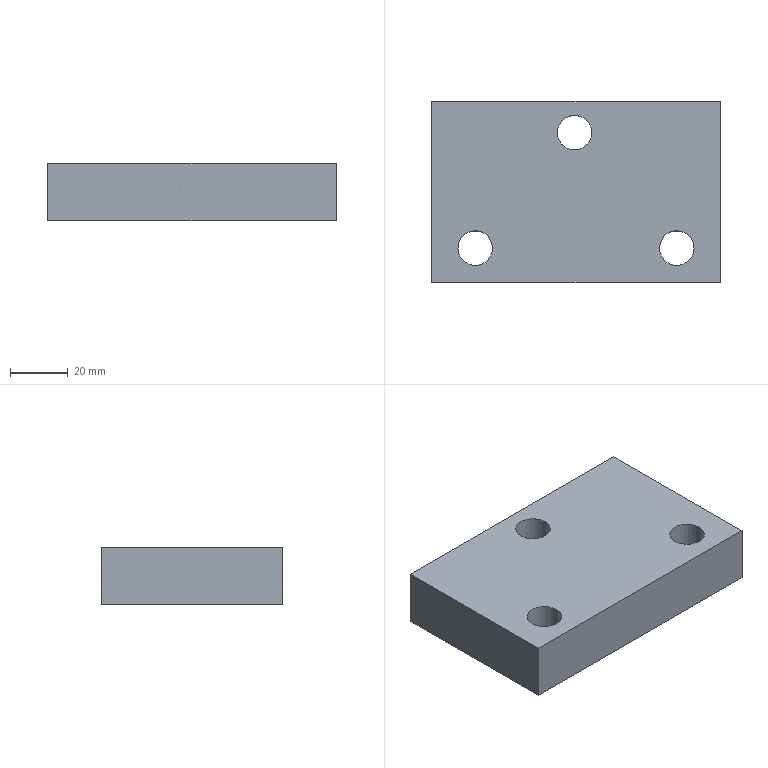Part | STEP file | cu dao nhan | 1 solid | 18 faces | box 100 x 63 x 20 mm | volume 110399 mm3 | plane 10 | cylinder 8 | commonest cylinder face diameters 12 x6 6 x2
STEP:
#1=CARTESIAN_POINT('',(0.,0.,0.));
#2=DIRECTION('',(0.,0.,1.));
#3=DIRECTION('',(1.,0.,0.));
#4=AXIS2_PLACEMENT_3D('',#1,#2,#3);
#5=CARTESIAN_POINT('',(55.5,52.1,5.));
#6=VERTEX_POINT('',#5);
#7=CARTESIAN_POINT('',(55.5,52.1,20.));
#8=VERTEX_POINT('',#7);
#9=CARTESIAN_POINT('',(55.5,52.1,-99.871));
#10=DIRECTION('',(0.,0.,1.));
#11=VECTOR('',#10,1.);
#12=LINE('',#9,#11);
#13=CARTESIAN_POINT('',(49.5,52.1,-99.871));
#14=DIRECTION('',(0.,0.,1.));
#15=DIRECTION('',(1.,0.,0.));
#16=AXIS2_PLACEMENT_3D('',#13,#14,#15);
#17=CYLINDRICAL_SURFACE('',#16,6.);
#18=CARTESIAN_POINT('',(6.283,0.));
#19=DIRECTION('',(0.,1.));
#20=VECTOR('',#19,1.);
#21=LINE('',#18,#20);
#22=(GEOMETRIC_REPRESENTATION_CONTEXT(2)PARAMETRIC_REPRESENTATION_CONTEXT()REPRESENTATION_CONTEXT('',''));
#23=DEFINITIONAL_REPRESENTATION('',(#21),#22);
#24=PCURVE('',#17,#23);
#25=CARTESIAN_POINT('',(49.5,52.1,-99.871));
#26=DIRECTION('',(0.,0.,1.));
#27=DIRECTION('',(1.,0.,0.));
#28=AXIS2_PLACEMENT_3D('',#25,#26,#27);
#29=CYLINDRICAL_SURFACE('',#28,6.);
#30=CARTESIAN_POINT('',(0.,0.));
#31=DIRECTION('',(0.,1.));
#32=VECTOR('',#31,1.);
#33=LINE('',#30,#32);
#34=(GEOMETRIC_REPRESENTATION_CONTEXT(2)PARAMETRIC_REPRESENTATION_CONTEXT()REPRESENTATION_CONTEXT('',''));
#35=DEFINITIONAL_REPRESENTATION('',(#33),#34);
#36=PCURVE('',#29,#35);
#37=SURFACE_CURVE('',#12,(#24,#36),.PCURVE_S1.);
#38=EDGE_CURVE('',#6,#8,#37,.T.);
#39=ORIENTED_EDGE('',*,*,#38,.T.);
#40=CARTESIAN_POINT('',(43.5,52.1,20.));
#41=VERTEX_POINT('',#40);
#42=CARTESIAN_POINT('',(49.5,52.1,20.));
#43=DIRECTION('',(0.,0.,-1.));
#44=DIRECTION('',(1.,0.,0.));
#45=AXIS2_PLACEMENT_3D('',#42,#43,#44);
#46=CIRCLE('',#45,6.);
#47=CARTESIAN_POINT('',(6.283,119.871));
#48=DIRECTION('',(-1.,0.));
#49=VECTOR('',#48,1.);
#50=LINE('',#47,#49);
#51=(GEOMETRIC_REPRESENTATION_CONTEXT(2)PARAMETRIC_REPRESENTATION_CONTEXT()REPRESENTATION_CONTEXT('',''));
#52=DEFINITIONAL_REPRESENTATION('',(#50),#51);
#53=PCURVE('',#17,#52);
#54=CARTESIAN_POINT('',(50.,31.5,20.));
#55=DIRECTION('',(0.,0.,1.));
#56=DIRECTION('',(1.,0.,0.));
#57=AXIS2_PLACEMENT_3D('',#54,#55,#56);
#58=PLANE('',#57);
#59=CARTESIAN_POINT('',(5.5,20.6));
#60=CARTESIAN_POINT('',(5.5,10.208));
#61=CARTESIAN_POINT('',(-3.5,15.404));
#62=CARTESIAN_POINT('',(-12.5,20.6));
#63=CARTESIAN_POINT('',(-3.5,25.796));
#64=CARTESIAN_POINT('',(5.5,30.992));
#65=CARTESIAN_POINT('',(5.5,20.6));
#66=(BOUNDED_CURVE()B_SPLINE_CURVE(2,(#59,#60,#61,#62,#63,#64,#65),.UNSPECIFIED.,.T.,.F.)B_SPLINE_CURVE_WITH_KNOTS((1,2,2,2,2,1),(-2.094,0.,2.094,4.189,6.283,8.378),.UNSPECIFIED.)CURVE()GEOMETRIC_REPRESENTATION_ITEM()RATIONAL_B_SPLINE_CURVE((1.,0.5,1.,0.5,1.,0.5,1.))REPRESENTATION_ITEM(''));
#67=(GEOMETRIC_REPRESENTATION_CONTEXT(2)PARAMETRIC_REPRESENTATION_CONTEXT()REPRESENTATION_CONTEXT('',''));
#68=DEFINITIONAL_REPRESENTATION('',(#66),#67);
#69=PCURVE('',#58,#68);
#70=SURFACE_CURVE('',#46,(#53,#69),.PCURVE_S1.);
#71=EDGE_CURVE('',#8,#41,#70,.T.);
#72=ORIENTED_EDGE('',*,*,#71,.T.);
#73=CARTESIAN_POINT('',(43.5,52.1,5.));
#74=VERTEX_POINT('',#73);
#75=CARTESIAN_POINT('',(43.5,52.1,-99.871));
#76=DIRECTION('',(0.,0.,1.));
#77=VECTOR('',#76,1.);
#78=LINE('',#75,#77);
#79=CARTESIAN_POINT('',(3.142,0.));
#80=DIRECTION('',(0.,1.));
#81=VECTOR('',#80,1.);
#82=LINE('',#79,#81);
#83=(GEOMETRIC_REPRESENTATION_CONTEXT(2)PARAMETRIC_REPRESENTATION_CONTEXT()REPRESENTATION_CONTEXT('',''));
#84=DEFINITIONAL_REPRESENTATION('',(#82),#83);
#85=PCURVE('',#17,#84);
#86=CARTESIAN_POINT('',(3.142,0.));
#87=DIRECTION('',(0.,1.));
#88=VECTOR('',#87,1.);
#89=LINE('',#86,#88);
#90=(GEOMETRIC_REPRESENTATION_CONTEXT(2)PARAMETRIC_REPRESENTATION_CONTEXT()REPRESENTATION_CONTEXT('',''));
#91=DEFINITIONAL_REPRESENTATION('',(#89),#90);
#92=PCURVE('',#29,#91);
#93=SURFACE_CURVE('',#78,(#85,#92),.PCURVE_S1.);
#94=EDGE_CURVE('',#74,#41,#93,.T.);
#95=ORIENTED_EDGE('',*,*,#94,.F.);
#96=CARTESIAN_POINT('',(49.5,52.1,5.));
#97=DIRECTION('',(0.,0.,1.));
#98=DIRECTION('',(1.,0.,0.));
#99=AXIS2_PLACEMENT_3D('',#96,#97,#98);
#100=CIRCLE('',#99,6.);
#101=CARTESIAN_POINT('',(0.,104.871));
#102=DIRECTION('',(1.,0.));
#103=VECTOR('',#102,1.);
#104=LINE('',#101,#103);
#105=(GEOMETRIC_REPRESENTATION_CONTEXT(2)PARAMETRIC_REPRESENTATION_CONTEXT()REPRESENTATION_CONTEXT('',''));
#106=DEFINITIONAL_REPRESENTATION('',(#104),#105);
#107=PCURVE('',#17,#106);
#108=CARTESIAN_POINT('',(26.,63.,5.));
#109=DIRECTION('',(0.,0.,1.));
#110=DIRECTION('',(1.,0.,0.));
#111=AXIS2_PLACEMENT_3D('',#108,#109,#110);
#112=PLANE('',#111);
#113=CARTESIAN_POINT('',(23.5,-10.9));
#114=DIRECTION('',(1.,0.));
#115=AXIS2_PLACEMENT_2D('',#113,#114);
#116=CIRCLE('',#115,6.);
#117=(GEOMETRIC_REPRESENTATION_CONTEXT(2)PARAMETRIC_REPRESENTATION_CONTEXT()REPRESENTATION_CONTEXT('',''));
#118=DEFINITIONAL_REPRESENTATION('',(#116),#117);
#119=PCURVE('',#112,#118);
#120=SURFACE_CURVE('',#100,(#107,#119),.PCURVE_S1.);
#121=EDGE_CURVE('',#74,#6,#120,.T.);
#122=ORIENTED_EDGE('',*,*,#121,.T.);
#123=EDGE_LOOP('',(#39,#72,#95,#122));
#124=FACE_BOUND('',#123,.F.);
#125=ADVANCED_FACE('',(#124),#17,.F.);
#126=CARTESIAN_POINT('',(21.,12.,0.));
#127=VERTEX_POINT('',#126);
#128=CARTESIAN_POINT('',(21.,12.,20.));
#129=VERTEX_POINT('',#128);
#130=CARTESIAN_POINT('',(21.,12.,-99.871));
#131=DIRECTION('',(0.,0.,1.));
#132=VECTOR('',#131,1.);
#133=LINE('',#130,#132);
#134=CARTESIAN_POINT('',(15.,12.,-99.871));
#135=DIRECTION('',(0.,0.,1.));
#136=DIRECTION('',(1.,0.,0.));
#137=AXIS2_PLACEMENT_3D('',#134,#135,#136);
#138=CYLINDRICAL_SURFACE('',#137,6.);
#139=CARTESIAN_POINT('',(6.283,0.));
#140=DIRECTION('',(0.,1.));
#141=VECTOR('',#140,1.);
#142=LINE('',#139,#141);
#143=(GEOMETRIC_REPRESENTATION_CONTEXT(2)PARAMETRIC_REPRESENTATION_CONTEXT()REPRESENTATION_CONTEXT('',''));
#144=DEFINITIONAL_REPRESENTATION('',(#142),#143);
#145=PCURVE('',#138,#144);
#146=CARTESIAN_POINT('',(15.,12.,-99.871));
#147=DIRECTION('',(0.,0.,1.));
#148=DIRECTION('',(1.,0.,0.));
#149=AXIS2_PLACEMENT_3D('',#146,#147,#148);
#150=CYLINDRICAL_SURFACE('',#149,6.);
#151=CARTESIAN_POINT('',(0.,0.));
#152=DIRECTION('',(0.,1.));
#153=VECTOR('',#152,1.);
#154=LINE('',#151,#153);
#155=(GEOMETRIC_REPRESENTATION_CONTEXT(2)PARAMETRIC_REPRESENTATION_CONTEXT()REPRESENTATION_CONTEXT('',''));
#156=DEFINITIONAL_REPRESENTATION('',(#154),#155);
#157=PCURVE('',#150,#156);
#158=SURFACE_CURVE('',#133,(#145,#157),.PCURVE_S1.);
#159=EDGE_CURVE('',#127,#129,#158,.T.);
#160=ORIENTED_EDGE('',*,*,#159,.T.);
#161=CARTESIAN_POINT('',(9.,12.,20.));
#162=VERTEX_POINT('',#161);
#163=CARTESIAN_POINT('',(15.,12.,20.));
#164=DIRECTION('',(0.,0.,-1.));
#165=DIRECTION('',(1.,0.,0.));
#166=AXIS2_PLACEMENT_3D('',#163,#164,#165);
#167=CIRCLE('',#166,6.);
#168=CARTESIAN_POINT('',(6.283,119.871));
#169=DIRECTION('',(-1.,0.));
#170=VECTOR('',#169,1.);
#171=LINE('',#168,#170);
#172=(GEOMETRIC_REPRESENTATION_CONTEXT(2)PARAMETRIC_REPRESENTATION_CONTEXT()REPRESENTATION_CONTEXT('',''));
#173=DEFINITIONAL_REPRESENTATION('',(#171),#172);
#174=PCURVE('',#138,#173);
#175=CARTESIAN_POINT('',(-29.,-19.5));
#176=CARTESIAN_POINT('',(-29.,-29.892));
#177=CARTESIAN_POINT('',(-38.,-24.696));
#178=CARTESIAN_POINT('',(-47.,-19.5));
#179=CARTESIAN_POINT('',(-38.,-14.304));
#180=CARTESIAN_POINT('',(-29.,-9.108));
#181=CARTESIAN_POINT('',(-29.,-19.5));
#182=(BOUNDED_CURVE()B_SPLINE_CURVE(2,(#175,#176,#177,#178,#179,#180,#181),.UNSPECIFIED.,.T.,.F.)B_SPLINE_CURVE_WITH_KNOTS((1,2,2,2,2,1),(-2.094,0.,2.094,4.189,6.283,8.378),.UNSPECIFIED.)CURVE()GEOMETRIC_REPRESENTATION_ITEM()RATIONAL_B_SPLINE_CURVE((1.,0.5,1.,0.5,1.,0.5,1.))REPRESENTATION_ITEM(''));
#183=(GEOMETRIC_REPRESENTATION_CONTEXT(2)PARAMETRIC_REPRESENTATION_CONTEXT()REPRESENTATION_CONTEXT('',''));
#184=DEFINITIONAL_REPRESENTATION('',(#182),#183);
#185=PCURVE('',#58,#184);
#186=SURFACE_CURVE('',#167,(#174,#185),.PCURVE_S1.);
#187=EDGE_CURVE('',#129,#162,#186,.T.);
#188=ORIENTED_EDGE('',*,*,#187,.T.);
#189=CARTESIAN_POINT('',(9.,12.,0.));
#190=VERTEX_POINT('',#189);
#191=CARTESIAN_POINT('',(9.,12.,-99.871));
#192=DIRECTION('',(0.,0.,1.));
#193=VECTOR('',#192,1.);
#194=LINE('',#191,#193);
#195=CARTESIAN_POINT('',(3.142,0.));
#196=DIRECTION('',(0.,1.));
#197=VECTOR('',#196,1.);
#198=LINE('',#195,#197);
#199=(GEOMETRIC_REPRESENTATION_CONTEXT(2)PARAMETRIC_REPRESENTATION_CONTEXT()REPRESENTATION_CONTEXT('',''));
#200=DEFINITIONAL_REPRESENTATION('',(#198),#199);
#201=PCURVE('',#138,#200);
#202=CARTESIAN_POINT('',(3.142,0.));
#203=DIRECTION('',(0.,1.));
#204=VECTOR('',#203,1.);
#205=LINE('',#202,#204);
#206=(GEOMETRIC_REPRESENTATION_CONTEXT(2)PARAMETRIC_REPRESENTATION_CONTEXT()REPRESENTATION_CONTEXT('',''));
#207=DEFINITIONAL_REPRESENTATION('',(#205),#206);
#208=PCURVE('',#150,#207);
#209=SURFACE_CURVE('',#194,(#201,#208),.PCURVE_S1.);
#210=EDGE_CURVE('',#190,#162,#209,.T.);
#211=ORIENTED_EDGE('',*,*,#210,.F.);
#212=CARTESIAN_POINT('',(15.,12.,0.));
#213=DIRECTION('',(0.,0.,1.));
#214=DIRECTION('',(1.,0.,0.));
#215=AXIS2_PLACEMENT_3D('',#212,#213,#214);
#216=CIRCLE('',#215,6.);
#217=CARTESIAN_POINT('',(0.,99.871));
#218=DIRECTION('',(1.,0.));
#219=VECTOR('',#218,1.);
#220=LINE('',#217,#219);
#221=(GEOMETRIC_REPRESENTATION_CONTEXT(2)PARAMETRIC_REPRESENTATION_CONTEXT()REPRESENTATION_CONTEXT('',''));
#222=DEFINITIONAL_REPRESENTATION('',(#220),#221);
#223=PCURVE('',#138,#222);
#224=CARTESIAN_POINT('',(50.,31.5,0.));
#225=DIRECTION('',(0.,0.,1.));
#226=DIRECTION('',(1.,0.,0.));
#227=AXIS2_PLACEMENT_3D('',#224,#225,#226);
#228=PLANE('',#227);
#229=CARTESIAN_POINT('',(-35.,-19.5));
#230=DIRECTION('',(1.,0.));
#231=AXIS2_PLACEMENT_2D('',#229,#230);
#232=CIRCLE('',#231,6.);
#233=(GEOMETRIC_REPRESENTATION_CONTEXT(2)PARAMETRIC_REPRESENTATION_CONTEXT()REPRESENTATION_CONTEXT('',''));
#234=DEFINITIONAL_REPRESENTATION('',(#232),#233);
#235=PCURVE('',#228,#234);
#236=SURFACE_CURVE('',#216,(#223,#235),.PCURVE_S1.);
#237=EDGE_CURVE('',#190,#127,#236,.T.);
#238=ORIENTED_EDGE('',*,*,#237,.T.);
#239=EDGE_LOOP('',(#160,#188,#211,#238));
#240=FACE_BOUND('',#239,.F.);
#241=ADVANCED_FACE('',(#240),#138,.F.);
#242=CARTESIAN_POINT('',(91.,12.,0.));
#243=VERTEX_POINT('',#242);
#244=CARTESIAN_POINT('',(91.,12.,20.));
#245=VERTEX_POINT('',#244);
#246=CARTESIAN_POINT('',(91.,12.,-99.871));
#247=DIRECTION('',(0.,0.,1.));
#248=VECTOR('',#247,1.);
#249=LINE('',#246,#248);
#250=CARTESIAN_POINT('',(85.,12.,-99.871));
#251=DIRECTION('',(0.,0.,1.));
#252=DIRECTION('',(1.,0.,0.));
#253=AXIS2_PLACEMENT_3D('',#250,#251,#252);
#254=CYLINDRICAL_SURFACE('',#253,6.);
#255=CARTESIAN_POINT('',(6.283,0.));
#256=DIRECTION('',(0.,1.));
#257=VECTOR('',#256,1.);
#258=LINE('',#255,#257);
#259=(GEOMETRIC_REPRESENTATION_CONTEXT(2)PARAMETRIC_REPRESENTATION_CONTEXT()REPRESENTATION_CONTEXT('',''));
#260=DEFINITIONAL_REPRESENTATION('',(#258),#259);
#261=PCURVE('',#254,#260);
#262=CARTESIAN_POINT('',(85.,12.,-99.871));
#263=DIRECTION('',(0.,0.,1.));
#264=DIRECTION('',(1.,0.,0.));
#265=AXIS2_PLACEMENT_3D('',#262,#263,#264);
#266=CYLINDRICAL_SURFACE('',#265,6.);
#267=CARTESIAN_POINT('',(0.,0.));
#268=DIRECTION('',(0.,1.));
#269=VECTOR('',#268,1.);
#270=LINE('',#267,#269);
#271=(GEOMETRIC_REPRESENTATION_CONTEXT(2)PARAMETRIC_REPRESENTATION_CONTEXT()REPRESENTATION_CONTEXT('',''));
#272=DEFINITIONAL_REPRESENTATION('',(#270),#271);
#273=PCURVE('',#266,#272);
#274=SURFACE_CURVE('',#249,(#261,#273),.PCURVE_S1.);
#275=EDGE_CURVE('',#243,#245,#274,.T.);
#276=ORIENTED_EDGE('',*,*,#275,.T.);
#277=CARTESIAN_POINT('',(79.,12.,20.));
#278=VERTEX_POINT('',#277);
#279=CARTESIAN_POINT('',(85.,12.,20.));
#280=DIRECTION('',(0.,0.,-1.));
#281=DIRECTION('',(1.,0.,0.));
#282=AXIS2_PLACEMENT_3D('',#279,#280,#281);
#283=CIRCLE('',#282,6.);
#284=CARTESIAN_POINT('',(6.283,119.871));
#285=DIRECTION('',(-1.,0.));
#286=VECTOR('',#285,1.);
#287=LINE('',#284,#286);
#288=(GEOMETRIC_REPRESENTATION_CONTEXT(2)PARAMETRIC_REPRESENTATION_CONTEXT()REPRESENTATION_CONTEXT('',''));
#289=DEFINITIONAL_REPRESENTATION('',(#287),#288);
#290=PCURVE('',#254,#289);
#291=CARTESIAN_POINT('',(41.,-19.5));
#292=CARTESIAN_POINT('',(41.,-29.892));
#293=CARTESIAN_POINT('',(32.,-24.696));
#294=CARTESIAN_POINT('',(23.,-19.5));
#295=CARTESIAN_POINT('',(32.,-14.304));
#296=CARTESIAN_POINT('',(41.,-9.108));
#297=CARTESIAN_POINT('',(41.,-19.5));
#298=(BOUNDED_CURVE()B_SPLINE_CURVE(2,(#291,#292,#293,#294,#295,#296,#297),.UNSPECIFIED.,.T.,.F.)B_SPLINE_CURVE_WITH_KNOTS((1,2,2,2,2,1),(-2.094,0.,2.094,4.189,6.283,8.378),.UNSPECIFIED.)CURVE()GEOMETRIC_REPRESENTATION_ITEM()RATIONAL_B_SPLINE_CURVE((1.,0.5,1.,0.5,1.,0.5,1.))REPRESENTATION_ITEM(''));
#299=(GEOMETRIC_REPRESENTATION_CONTEXT(2)PARAMETRIC_REPRESENTATION_CONTEXT()REPRESENTATION_CONTEXT('',''));
#300=DEFINITIONAL_REPRESENTATION('',(#298),#299);
#301=PCURVE('',#58,#300);
#302=SURFACE_CURVE('',#283,(#290,#301),.PCURVE_S1.);
#303=EDGE_CURVE('',#245,#278,#302,.T.);
#304=ORIENTED_EDGE('',*,*,#303,.T.);
#305=CARTESIAN_POINT('',(79.,12.,0.));
#306=VERTEX_POINT('',#305);
#307=CARTESIAN_POINT('',(79.,12.,-99.871));
#308=DIRECTION('',(0.,0.,1.));
#309=VECTOR('',#308,1.);
#310=LINE('',#307,#309);
#311=CARTESIAN_POINT('',(3.142,0.));
#312=DIRECTION('',(0.,1.));
#313=VECTOR('',#312,1.);
#314=LINE('',#311,#313);
#315=(GEOMETRIC_REPRESENTATION_CONTEXT(2)PARAMETRIC_REPRESENTATION_CONTEXT()REPRESENTATION_CONTEXT('',''));
#316=DEFINITIONAL_REPRESENTATION('',(#314),#315);
#317=PCURVE('',#254,#316);
#318=CARTESIAN_POINT('',(3.142,0.));
#319=DIRECTION('',(0.,1.));
#320=VECTOR('',#319,1.);
#321=LINE('',#318,#320);
#322=(GEOMETRIC_REPRESENTATION_CONTEXT(2)PARAMETRIC_REPRESENTATION_CONTEXT()REPRESENTATION_CONTEXT('',''));
#323=DEFINITIONAL_REPRESENTATION('',(#321),#322);
#324=PCURVE('',#266,#323);
#325=SURFACE_CURVE('',#310,(#317,#324),.PCURVE_S1.);
#326=EDGE_CURVE('',#306,#278,#325,.T.);
#327=ORIENTED_EDGE('',*,*,#326,.F.);
#328=CARTESIAN_POINT('',(85.,12.,0.));
#329=DIRECTION('',(0.,0.,1.));
#330=DIRECTION('',(1.,0.,0.));
#331=AXIS2_PLACEMENT_3D('',#328,#329,#330);
#332=CIRCLE('',#331,6.);
#333=CARTESIAN_POINT('',(0.,99.871));
#334=DIRECTION('',(1.,0.));
#335=VECTOR('',#334,1.);
#336=LINE('',#333,#335);
#337=(GEOMETRIC_REPRESENTATION_CONTEXT(2)PARAMETRIC_REPRESENTATION_CONTEXT()REPRESENTATION_CONTEXT('',''));
#338=DEFINITIONAL_REPRESENTATION('',(#336),#337);
#339=PCURVE('',#254,#338);
#340=CARTESIAN_POINT('',(35.,-19.5));
#341=DIRECTION('',(1.,0.));
#342=AXIS2_PLACEMENT_2D('',#340,#341);
#343=CIRCLE('',#342,6.);
#344=(GEOMETRIC_REPRESENTATION_CONTEXT(2)PARAMETRIC_REPRESENTATION_CONTEXT()REPRESENTATION_CONTEXT('',''));
#345=DEFINITIONAL_REPRESENTATION('',(#343),#344);
#346=PCURVE('',#228,#345);
#347=SURFACE_CURVE('',#332,(#339,#346),.PCURVE_S1.);
#348=EDGE_CURVE('',#306,#243,#347,.T.);
#349=ORIENTED_EDGE('',*,*,#348,.T.);
#350=EDGE_LOOP('',(#276,#304,#327,#349));
#351=FACE_BOUND('',#350,.F.);
#352=ADVANCED_FACE('',(#351),#254,.F.);
#353=ORIENTED_EDGE('',*,*,#71,.T.);
#354=CARTESIAN_POINT('',(49.5,52.1,20.));
#355=DIRECTION('',(0.,0.,-1.));
#356=DIRECTION('',(1.,0.,0.));
#357=AXIS2_PLACEMENT_3D('',#354,#355,#356);
#358=CIRCLE('',#357,6.);
#359=CARTESIAN_POINT('',(5.5,20.6));
#360=CARTESIAN_POINT('',(5.5,10.208));
#361=CARTESIAN_POINT('',(-3.5,15.404));
#362=CARTESIAN_POINT('',(-12.5,20.6));
#363=CARTESIAN_POINT('',(-3.5,25.796));
#364=CARTESIAN_POINT('',(5.5,30.992));
#365=CARTESIAN_POINT('',(5.5,20.6));
#366=(BOUNDED_CURVE()B_SPLINE_CURVE(2,(#359,#360,#361,#362,#363,#364,#365),.UNSPECIFIED.,.T.,.F.)B_SPLINE_CURVE_WITH_KNOTS((1,2,2,2,2,1),(-2.094,0.,2.094,4.189,6.283,8.378),.UNSPECIFIED.)CURVE()GEOMETRIC_REPRESENTATION_ITEM()RATIONAL_B_SPLINE_CURVE((1.,0.5,1.,0.5,1.,0.5,1.))REPRESENTATION_ITEM(''));
#367=(GEOMETRIC_REPRESENTATION_CONTEXT(2)PARAMETRIC_REPRESENTATION_CONTEXT()REPRESENTATION_CONTEXT('',''));
#368=DEFINITIONAL_REPRESENTATION('',(#366),#367);
#369=PCURVE('',#58,#368);
#370=CARTESIAN_POINT('',(6.283,119.871));
#371=DIRECTION('',(-1.,0.));
#372=VECTOR('',#371,1.);
#373=LINE('',#370,#372);
#374=(GEOMETRIC_REPRESENTATION_CONTEXT(2)PARAMETRIC_REPRESENTATION_CONTEXT()REPRESENTATION_CONTEXT('',''));
#375=DEFINITIONAL_REPRESENTATION('',(#373),#374);
#376=PCURVE('',#29,#375);
#377=SURFACE_CURVE('',#358,(#369,#376),.PCURVE_S1.);
#378=EDGE_CURVE('',#41,#8,#377,.T.);
#379=ORIENTED_EDGE('',*,*,#378,.T.);
#380=EDGE_LOOP('',(#353,#379));
#381=FACE_BOUND('',#380,.T.);
#382=ORIENTED_EDGE('',*,*,#187,.T.);
#383=CARTESIAN_POINT('',(15.,12.,20.));
#384=DIRECTION('',(0.,0.,-1.));
#385=DIRECTION('',(1.,0.,0.));
#386=AXIS2_PLACEMENT_3D('',#383,#384,#385);
#387=CIRCLE('',#386,6.);
#388=CARTESIAN_POINT('',(-29.,-19.5));
#389=CARTESIAN_POINT('',(-29.,-29.892));
#390=CARTESIAN_POINT('',(-38.,-24.696));
#391=CARTESIAN_POINT('',(-47.,-19.5));
#392=CARTESIAN_POINT('',(-38.,-14.304));
#393=CARTESIAN_POINT('',(-29.,-9.108));
#394=CARTESIAN_POINT('',(-29.,-19.5));
#395=(BOUNDED_CURVE()B_SPLINE_CURVE(2,(#388,#389,#390,#391,#392,#393,#394),.UNSPECIFIED.,.T.,.F.)B_SPLINE_CURVE_WITH_KNOTS((1,2,2,2,2,1),(-2.094,0.,2.094,4.189,6.283,8.378),.UNSPECIFIED.)CURVE()GEOMETRIC_REPRESENTATION_ITEM()RATIONAL_B_SPLINE_CURVE((1.,0.5,1.,0.5,1.,0.5,1.))REPRESENTATION_ITEM(''));
#396=(GEOMETRIC_REPRESENTATION_CONTEXT(2)PARAMETRIC_REPRESENTATION_CONTEXT()REPRESENTATION_CONTEXT('',''));
#397=DEFINITIONAL_REPRESENTATION('',(#395),#396);
#398=PCURVE('',#58,#397);
#399=CARTESIAN_POINT('',(6.283,119.871));
#400=DIRECTION('',(-1.,0.));
#401=VECTOR('',#400,1.);
#402=LINE('',#399,#401);
#403=(GEOMETRIC_REPRESENTATION_CONTEXT(2)PARAMETRIC_REPRESENTATION_CONTEXT()REPRESENTATION_CONTEXT('',''));
#404=DEFINITIONAL_REPRESENTATION('',(#402),#403);
#405=PCURVE('',#150,#404);
#406=SURFACE_CURVE('',#387,(#398,#405),.PCURVE_S1.);
#407=EDGE_CURVE('',#162,#129,#406,.T.);
#408=ORIENTED_EDGE('',*,*,#407,.T.);
#409=EDGE_LOOP('',(#382,#408));
#410=FACE_BOUND('',#409,.T.);
#411=ORIENTED_EDGE('',*,*,#303,.T.);
#412=CARTESIAN_POINT('',(85.,12.,20.));
#413=DIRECTION('',(0.,0.,-1.));
#414=DIRECTION('',(1.,0.,0.));
#415=AXIS2_PLACEMENT_3D('',#412,#413,#414);
#416=CIRCLE('',#415,6.);
#417=CARTESIAN_POINT('',(41.,-19.5));
#418=CARTESIAN_POINT('',(41.,-29.892));
#419=CARTESIAN_POINT('',(32.,-24.696));
#420=CARTESIAN_POINT('',(23.,-19.5));
#421=CARTESIAN_POINT('',(32.,-14.304));
#422=CARTESIAN_POINT('',(41.,-9.108));
#423=CARTESIAN_POINT('',(41.,-19.5));
#424=(BOUNDED_CURVE()B_SPLINE_CURVE(2,(#417,#418,#419,#420,#421,#422,#423),.UNSPECIFIED.,.T.,.F.)B_SPLINE_CURVE_WITH_KNOTS((1,2,2,2,2,1),(-2.094,0.,2.094,4.189,6.283,8.378),.UNSPECIFIED.)CURVE()GEOMETRIC_REPRESENTATION_ITEM()RATIONAL_B_SPLINE_CURVE((1.,0.5,1.,0.5,1.,0.5,1.))REPRESENTATION_ITEM(''));
#425=(GEOMETRIC_REPRESENTATION_CONTEXT(2)PARAMETRIC_REPRESENTATION_CONTEXT()REPRESENTATION_CONTEXT('',''));
#426=DEFINITIONAL_REPRESENTATION('',(#424),#425);
#427=PCURVE('',#58,#426);
#428=CARTESIAN_POINT('',(6.283,119.871));
#429=DIRECTION('',(-1.,0.));
#430=VECTOR('',#429,1.);
#431=LINE('',#428,#430);
#432=(GEOMETRIC_REPRESENTATION_CONTEXT(2)PARAMETRIC_REPRESENTATION_CONTEXT()REPRESENTATION_CONTEXT('',''));
#433=DEFINITIONAL_REPRESENTATION('',(#431),#432);
#434=PCURVE('',#266,#433);
#435=SURFACE_CURVE('',#416,(#427,#434),.PCURVE_S1.);
#436=EDGE_CURVE('',#278,#245,#435,.T.);
#437=ORIENTED_EDGE('',*,*,#436,.T.);
#438=EDGE_LOOP('',(#411,#437));
#439=FACE_BOUND('',#438,.T.);
#440=CARTESIAN_POINT('',(100.,0.,20.));
#441=VERTEX_POINT('',#440);
#442=CARTESIAN_POINT('',(100.,63.,20.));
#443=VERTEX_POINT('',#442);
#444=CARTESIAN_POINT('',(100.,31.5,20.));
#445=DIRECTION('',(0.,1.,0.));
#446=VECTOR('',#445,1.);
#447=LINE('',#444,#446);
#448=CARTESIAN_POINT('',(50.,0.));
#449=DIRECTION('',(0.,1.));
#450=VECTOR('',#449,1.);
#451=LINE('',#448,#450);
#452=(GEOMETRIC_REPRESENTATION_CONTEXT(2)PARAMETRIC_REPRESENTATION_CONTEXT()REPRESENTATION_CONTEXT('',''));
#453=DEFINITIONAL_REPRESENTATION('',(#451),#452);
#454=PCURVE('',#58,#453);
#455=CARTESIAN_POINT('',(100.,63.,0.));
#456=DIRECTION('',(1.,0.,0.));
#457=DIRECTION('',(0.,0.,-1.));
#458=AXIS2_PLACEMENT_3D('',#455,#456,#457);
#459=PLANE('',#458);
#460=CARTESIAN_POINT('',(-20.,-31.5));
#461=DIRECTION('',(0.,1.));
#462=VECTOR('',#461,1.);
#463=LINE('',#460,#462);
#464=(GEOMETRIC_REPRESENTATION_CONTEXT(2)PARAMETRIC_REPRESENTATION_CONTEXT()REPRESENTATION_CONTEXT('',''));
#465=DEFINITIONAL_REPRESENTATION('',(#463),#464);
#466=PCURVE('',#459,#465);
#467=SURFACE_CURVE('',#447,(#454,#466),.PCURVE_S1.);
#468=EDGE_CURVE('',#441,#443,#467,.T.);
#469=ORIENTED_EDGE('',*,*,#468,.T.);
#470=CARTESIAN_POINT('',(0.,63.,20.));
#471=VERTEX_POINT('',#470);
#472=CARTESIAN_POINT('',(50.,63.,20.));
#473=DIRECTION('',(-1.,0.,0.));
#474=VECTOR('',#473,1.);
#475=LINE('',#472,#474);
#476=CARTESIAN_POINT('',(0.,31.5));
#477=DIRECTION('',(-1.,0.));
#478=VECTOR('',#477,1.);
#479=LINE('',#476,#478);
#480=(GEOMETRIC_REPRESENTATION_CONTEXT(2)PARAMETRIC_REPRESENTATION_CONTEXT()REPRESENTATION_CONTEXT('',''));
#481=DEFINITIONAL_REPRESENTATION('',(#479),#480);
#482=PCURVE('',#58,#481);
#483=CARTESIAN_POINT('',(0.,63.,0.));
#484=DIRECTION('',(0.,1.,0.));
#485=DIRECTION('',(0.,0.,1.));
#486=AXIS2_PLACEMENT_3D('',#483,#484,#485);
#487=PLANE('',#486);
#488=CARTESIAN_POINT('',(20.,50.));
#489=DIRECTION('',(0.,-1.));
#490=VECTOR('',#489,1.);
#491=LINE('',#488,#490);
#492=(GEOMETRIC_REPRESENTATION_CONTEXT(2)PARAMETRIC_REPRESENTATION_CONTEXT()REPRESENTATION_CONTEXT('',''));
#493=DEFINITIONAL_REPRESENTATION('',(#491),#492);
#494=PCURVE('',#487,#493);
#495=SURFACE_CURVE('',#475,(#482,#494),.PCURVE_S1.);
#496=EDGE_CURVE('',#443,#471,#495,.T.);
#497=ORIENTED_EDGE('',*,*,#496,.T.);
#498=CARTESIAN_POINT('',(0.,0.,20.));
#499=VERTEX_POINT('',#498);
#500=CARTESIAN_POINT('',(0.,31.5,20.));
#501=DIRECTION('',(0.,-1.,0.));
#502=VECTOR('',#501,1.);
#503=LINE('',#500,#502);
#504=CARTESIAN_POINT('',(-50.,0.));
#505=DIRECTION('',(0.,-1.));
#506=VECTOR('',#505,1.);
#507=LINE('',#504,#506);
#508=(GEOMETRIC_REPRESENTATION_CONTEXT(2)PARAMETRIC_REPRESENTATION_CONTEXT()REPRESENTATION_CONTEXT('',''));
#509=DEFINITIONAL_REPRESENTATION('',(#507),#508);
#510=PCURVE('',#58,#509);
#511=CARTESIAN_POINT('',(0.,0.,0.));
#512=DIRECTION('',(-1.,0.,0.));
#513=DIRECTION('',(0.,0.,1.));
#514=AXIS2_PLACEMENT_3D('',#511,#512,#513);
#515=PLANE('',#514);
#516=CARTESIAN_POINT('',(20.,31.5));
#517=DIRECTION('',(0.,-1.));
#518=VECTOR('',#517,1.);
#519=LINE('',#516,#518);
#520=(GEOMETRIC_REPRESENTATION_CONTEXT(2)PARAMETRIC_REPRESENTATION_CONTEXT()REPRESENTATION_CONTEXT('',''));
#521=DEFINITIONAL_REPRESENTATION('',(#519),#520);
#522=PCURVE('',#515,#521);
#523=SURFACE_CURVE('',#503,(#510,#522),.PCURVE_S1.);
#524=EDGE_CURVE('',#471,#499,#523,.T.);
#525=ORIENTED_EDGE('',*,*,#524,.T.);
#526=CARTESIAN_POINT('',(50.,0.,20.));
#527=DIRECTION('',(1.,0.,0.));
#528=VECTOR('',#527,1.);
#529=LINE('',#526,#528);
#530=CARTESIAN_POINT('',(0.,-31.5));
#531=DIRECTION('',(1.,0.));
#532=VECTOR('',#531,1.);
#533=LINE('',#530,#532);
#534=(GEOMETRIC_REPRESENTATION_CONTEXT(2)PARAMETRIC_REPRESENTATION_CONTEXT()REPRESENTATION_CONTEXT('',''));
#535=DEFINITIONAL_REPRESENTATION('',(#533),#534);
#536=PCURVE('',#58,#535);
#537=CARTESIAN_POINT('',(100.,0.,0.));
#538=DIRECTION('',(0.,-1.,0.));
#539=DIRECTION('',(0.,0.,-1.));
#540=AXIS2_PLACEMENT_3D('',#537,#538,#539);
#541=PLANE('',#540);
#542=CARTESIAN_POINT('',(-20.,-50.));
#543=DIRECTION('',(0.,1.));
#544=VECTOR('',#543,1.);
#545=LINE('',#542,#544);
#546=(GEOMETRIC_REPRESENTATION_CONTEXT(2)PARAMETRIC_REPRESENTATION_CONTEXT()REPRESENTATION_CONTEXT('',''));
#547=DEFINITIONAL_REPRESENTATION('',(#545),#546);
#548=PCURVE('',#541,#547);
#549=SURFACE_CURVE('',#529,(#536,#548),.PCURVE_S1.);
#550=EDGE_CURVE('',#499,#441,#549,.T.);
#551=ORIENTED_EDGE('',*,*,#550,.T.);
#552=EDGE_LOOP('',(#469,#497,#525,#551));
#553=FACE_BOUND('',#552,.T.);
#554=ADVANCED_FACE('',(#381,#410,#439,#553),#58,.T.);
#555=ORIENTED_EDGE('',*,*,#378,.T.);
#556=ORIENTED_EDGE('',*,*,#38,.F.);
#557=CARTESIAN_POINT('',(49.5,52.1,5.));
#558=DIRECTION('',(0.,0.,1.));
#559=DIRECTION('',(1.,0.,0.));
#560=AXIS2_PLACEMENT_3D('',#557,#558,#559);
#561=CIRCLE('',#560,6.);
#562=CARTESIAN_POINT('',(0.,104.871));
#563=DIRECTION('',(1.,0.));
#564=VECTOR('',#563,1.);
#565=LINE('',#562,#564);
#566=(GEOMETRIC_REPRESENTATION_CONTEXT(2)PARAMETRIC_REPRESENTATION_CONTEXT()REPRESENTATION_CONTEXT('',''));
#567=DEFINITIONAL_REPRESENTATION('',(#565),#566);
#568=PCURVE('',#29,#567);
#569=CARTESIAN_POINT('',(23.5,-10.9));
#570=DIRECTION('',(1.,0.));
#571=AXIS2_PLACEMENT_2D('',#569,#570);
#572=CIRCLE('',#571,6.);
#573=(GEOMETRIC_REPRESENTATION_CONTEXT(2)PARAMETRIC_REPRESENTATION_CONTEXT()REPRESENTATION_CONTEXT('',''));
#574=DEFINITIONAL_REPRESENTATION('',(#572),#573);
#575=PCURVE('',#112,#574);
#576=SURFACE_CURVE('',#561,(#568,#575),.PCURVE_S1.);
#577=EDGE_CURVE('',#6,#74,#576,.T.);
#578=ORIENTED_EDGE('',*,*,#577,.T.);
#579=ORIENTED_EDGE('',*,*,#94,.T.);
#580=EDGE_LOOP('',(#555,#556,#578,#579));
#581=FACE_BOUND('',#580,.F.);
#582=ADVANCED_FACE('',(#581),#29,.F.);
#583=ORIENTED_EDGE('',*,*,#407,.T.);
#584=ORIENTED_EDGE('',*,*,#159,.F.);
#585=CARTESIAN_POINT('',(15.,12.,0.));
#586=DIRECTION('',(0.,0.,1.));
#587=DIRECTION('',(1.,0.,0.));
#588=AXIS2_PLACEMENT_3D('',#585,#586,#587);
#589=CIRCLE('',#588,6.);
#590=CARTESIAN_POINT('',(0.,99.871));
#591=DIRECTION('',(1.,0.));
#592=VECTOR('',#591,1.);
#593=LINE('',#590,#592);
#594=(GEOMETRIC_REPRESENTATION_CONTEXT(2)PARAMETRIC_REPRESENTATION_CONTEXT()REPRESENTATION_CONTEXT('',''));
#595=DEFINITIONAL_REPRESENTATION('',(#593),#594);
#596=PCURVE('',#150,#595);
#597=CARTESIAN_POINT('',(-35.,-19.5));
#598=DIRECTION('',(1.,0.));
#599=AXIS2_PLACEMENT_2D('',#597,#598);
#600=CIRCLE('',#599,6.);
#601=(GEOMETRIC_REPRESENTATION_CONTEXT(2)PARAMETRIC_REPRESENTATION_CONTEXT()REPRESENTATION_CONTEXT('',''));
#602=DEFINITIONAL_REPRESENTATION('',(#600),#601);
#603=PCURVE('',#228,#602);
#604=SURFACE_CURVE('',#589,(#596,#603),.PCURVE_S1.);
#605=EDGE_CURVE('',#127,#190,#604,.T.);
#606=ORIENTED_EDGE('',*,*,#605,.T.);
#607=ORIENTED_EDGE('',*,*,#210,.T.);
#608=EDGE_LOOP('',(#583,#584,#606,#607));
#609=FACE_BOUND('',#608,.F.);
#610=ADVANCED_FACE('',(#609),#150,.F.);
#611=ORIENTED_EDGE('',*,*,#436,.T.);
#612=ORIENTED_EDGE('',*,*,#275,.F.);
#613=CARTESIAN_POINT('',(85.,12.,0.));
#614=DIRECTION('',(0.,0.,1.));
#615=DIRECTION('',(1.,0.,0.));
#616=AXIS2_PLACEMENT_3D('',#613,#614,#615);
#617=CIRCLE('',#616,6.);
#618=CARTESIAN_POINT('',(0.,99.871));
#619=DIRECTION('',(1.,0.));
#620=VECTOR('',#619,1.);
#621=LINE('',#618,#620);
#622=(GEOMETRIC_REPRESENTATION_CONTEXT(2)PARAMETRIC_REPRESENTATION_CONTEXT()REPRESENTATION_CONTEXT('',''));
#623=DEFINITIONAL_REPRESENTATION('',(#621),#622);
#624=PCURVE('',#266,#623);
#625=CARTESIAN_POINT('',(35.,-19.5));
#626=DIRECTION('',(1.,0.));
#627=AXIS2_PLACEMENT_2D('',#625,#626);
#628=CIRCLE('',#627,6.);
#629=(GEOMETRIC_REPRESENTATION_CONTEXT(2)PARAMETRIC_REPRESENTATION_CONTEXT()REPRESENTATION_CONTEXT('',''));
#630=DEFINITIONAL_REPRESENTATION('',(#628),#629);
#631=PCURVE('',#228,#630);
#632=SURFACE_CURVE('',#617,(#624,#631),.PCURVE_S1.);
#633=EDGE_CURVE('',#243,#306,#632,.T.);
#634=ORIENTED_EDGE('',*,*,#633,.T.);
#635=ORIENTED_EDGE('',*,*,#326,.T.);
#636=EDGE_LOOP('',(#611,#612,#634,#635));
#637=FACE_BOUND('',#636,.F.);
#638=ADVANCED_FACE('',(#637),#266,.F.);
#639=CARTESIAN_POINT('',(73.,63.,0.));
#640=VERTEX_POINT('',#639);
#641=CARTESIAN_POINT('',(73.,63.,5.));
#642=VERTEX_POINT('',#641);
#643=CARTESIAN_POINT('',(73.,63.,0.));
#644=DIRECTION('',(0.,0.,1.));
#645=VECTOR('',#644,1.);
#646=LINE('',#643,#645);
#647=CARTESIAN_POINT('',(0.,73.));
#648=DIRECTION('',(1.,0.));
#649=VECTOR('',#648,1.);
#650=LINE('',#647,#649);
#651=(GEOMETRIC_REPRESENTATION_CONTEXT(2)PARAMETRIC_REPRESENTATION_CONTEXT()REPRESENTATION_CONTEXT('',''));
#652=DEFINITIONAL_REPRESENTATION('',(#650),#651);
#653=PCURVE('',#487,#652);
#654=CARTESIAN_POINT('',(73.,63.,5.));
#655=DIRECTION('',(1.,0.,0.));
#656=DIRECTION('',(0.,0.,-1.));
#657=AXIS2_PLACEMENT_3D('',#654,#655,#656);
#658=PLANE('',#657);
#659=CARTESIAN_POINT('',(5.,0.));
#660=DIRECTION('',(-1.,0.));
#661=VECTOR('',#660,1.);
#662=LINE('',#659,#661);
#663=(GEOMETRIC_REPRESENTATION_CONTEXT(2)PARAMETRIC_REPRESENTATION_CONTEXT()REPRESENTATION_CONTEXT('',''));
#664=DEFINITIONAL_REPRESENTATION('',(#662),#663);
#665=PCURVE('',#658,#664);
#666=SURFACE_CURVE('',#646,(#653,#665),.PCURVE_S1.);
#667=EDGE_CURVE('',#640,#642,#666,.T.);
#668=ORIENTED_EDGE('',*,*,#667,.T.);
#669=CARTESIAN_POINT('',(26.,63.,5.));
#670=VERTEX_POINT('',#669);
#671=CARTESIAN_POINT('',(0.,63.,5.));
#672=DIRECTION('',(-1.,0.,0.));
#673=VECTOR('',#672,1.);
#674=LINE('',#671,#673);
#675=CARTESIAN_POINT('',(5.,0.));
#676=DIRECTION('',(0.,-1.));
#677=VECTOR('',#676,1.);
#678=LINE('',#675,#677);
#679=(GEOMETRIC_REPRESENTATION_CONTEXT(2)PARAMETRIC_REPRESENTATION_CONTEXT()REPRESENTATION_CONTEXT('',''));
#680=DEFINITIONAL_REPRESENTATION('',(#678),#679);
#681=PCURVE('',#487,#680);
#682=CARTESIAN_POINT('',(-26.,0.));
#683=DIRECTION('',(-1.,0.));
#684=VECTOR('',#683,1.);
#685=LINE('',#682,#684);
#686=(GEOMETRIC_REPRESENTATION_CONTEXT(2)PARAMETRIC_REPRESENTATION_CONTEXT()REPRESENTATION_CONTEXT('',''));
#687=DEFINITIONAL_REPRESENTATION('',(#685),#686);
#688=PCURVE('',#112,#687);
#689=SURFACE_CURVE('',#674,(#681,#688),.PCURVE_S1.);
#690=EDGE_CURVE('',#642,#670,#689,.T.);
#691=ORIENTED_EDGE('',*,*,#690,.T.);
#692=CARTESIAN_POINT('',(26.,63.,0.));
#693=VERTEX_POINT('',#692);
#694=CARTESIAN_POINT('',(26.,63.,0.));
#695=DIRECTION('',(0.,0.,-1.));
#696=VECTOR('',#695,1.);
#697=LINE('',#694,#696);
#698=CARTESIAN_POINT('',(0.,26.));
#699=DIRECTION('',(-1.,0.));
#700=VECTOR('',#699,1.);
#701=LINE('',#698,#700);
#702=(GEOMETRIC_REPRESENTATION_CONTEXT(2)PARAMETRIC_REPRESENTATION_CONTEXT()REPRESENTATION_CONTEXT('',''));
#703=DEFINITIONAL_REPRESENTATION('',(#701),#702);
#704=PCURVE('',#487,#703);
#705=CARTESIAN_POINT('',(26.,63.,0.));
#706=DIRECTION('',(-1.,0.,0.));
#707=DIRECTION('',(0.,0.,1.));
#708=AXIS2_PLACEMENT_3D('',#705,#706,#707);
#709=PLANE('',#708);
#710=CARTESIAN_POINT('',(0.,0.));
#711=DIRECTION('',(-1.,0.));
#712=VECTOR('',#711,1.);
#713=LINE('',#710,#712);
#714=(GEOMETRIC_REPRESENTATION_CONTEXT(2)PARAMETRIC_REPRESENTATION_CONTEXT()REPRESENTATION_CONTEXT('',''));
#715=DEFINITIONAL_REPRESENTATION('',(#713),#714);
#716=PCURVE('',#709,#715);
#717=SURFACE_CURVE('',#697,(#704,#716),.PCURVE_S1.);
#718=EDGE_CURVE('',#670,#693,#717,.T.);
#719=ORIENTED_EDGE('',*,*,#718,.T.);
#720=CARTESIAN_POINT('',(0.,63.,0.));
#721=VERTEX_POINT('',#720);
#722=CARTESIAN_POINT('',(0.,63.,0.));
#723=DIRECTION('',(-1.,0.,0.));
#724=VECTOR('',#723,1.);
#725=LINE('',#722,#724);
#726=CARTESIAN_POINT('',(0.,0.));
#727=DIRECTION('',(0.,-1.));
#728=VECTOR('',#727,1.);
#729=LINE('',#726,#728);
#730=(GEOMETRIC_REPRESENTATION_CONTEXT(2)PARAMETRIC_REPRESENTATION_CONTEXT()REPRESENTATION_CONTEXT('',''));
#731=DEFINITIONAL_REPRESENTATION('',(#729),#730);
#732=PCURVE('',#487,#731);
#733=CARTESIAN_POINT('',(-50.,31.5));
#734=DIRECTION('',(-1.,0.));
#735=VECTOR('',#734,1.);
#736=LINE('',#733,#735);
#737=(GEOMETRIC_REPRESENTATION_CONTEXT(2)PARAMETRIC_REPRESENTATION_CONTEXT()REPRESENTATION_CONTEXT('',''));
#738=DEFINITIONAL_REPRESENTATION('',(#736),#737);
#739=PCURVE('',#228,#738);
#740=SURFACE_CURVE('',#725,(#732,#739),.PCURVE_S1.);
#741=EDGE_CURVE('',#693,#721,#740,.T.);
#742=ORIENTED_EDGE('',*,*,#741,.T.);
#743=CARTESIAN_POINT('',(0.,63.,0.));
#744=DIRECTION('',(0.,0.,1.));
#745=VECTOR('',#744,1.);
#746=LINE('',#743,#745);
#747=CARTESIAN_POINT('',(0.,0.));
#748=DIRECTION('',(1.,0.));
#749=VECTOR('',#748,1.);
#750=LINE('',#747,#749);
#751=(GEOMETRIC_REPRESENTATION_CONTEXT(2)PARAMETRIC_REPRESENTATION_CONTEXT()REPRESENTATION_CONTEXT('',''));
#752=DEFINITIONAL_REPRESENTATION('',(#750),#751);
#753=PCURVE('',#487,#752);
#754=CARTESIAN_POINT('',(0.,63.));
#755=DIRECTION('',(1.,0.));
#756=VECTOR('',#755,1.);
#757=LINE('',#754,#756);
#758=(GEOMETRIC_REPRESENTATION_CONTEXT(2)PARAMETRIC_REPRESENTATION_CONTEXT()REPRESENTATION_CONTEXT('',''));
#759=DEFINITIONAL_REPRESENTATION('',(#757),#758);
#760=PCURVE('',#515,#759);
#761=SURFACE_CURVE('',#746,(#753,#760),.PCURVE_S1.);
#762=EDGE_CURVE('',#721,#471,#761,.T.);
#763=ORIENTED_EDGE('',*,*,#762,.T.);
#764=ORIENTED_EDGE('',*,*,#496,.F.);
#765=CARTESIAN_POINT('',(100.,63.,0.));
#766=VERTEX_POINT('',#765);
#767=CARTESIAN_POINT('',(100.,63.,0.));
#768=DIRECTION('',(0.,0.,-1.));
#769=VECTOR('',#768,1.);
#770=LINE('',#767,#769);
#771=CARTESIAN_POINT('',(0.,100.));
#772=DIRECTION('',(-1.,0.));
#773=VECTOR('',#772,1.);
#774=LINE('',#771,#773);
#775=(GEOMETRIC_REPRESENTATION_CONTEXT(2)PARAMETRIC_REPRESENTATION_CONTEXT()REPRESENTATION_CONTEXT('',''));
#776=DEFINITIONAL_REPRESENTATION('',(#774),#775);
#777=PCURVE('',#487,#776);
#778=CARTESIAN_POINT('',(0.,0.));
#779=DIRECTION('',(1.,0.));
#780=VECTOR('',#779,1.);
#781=LINE('',#778,#780);
#782=(GEOMETRIC_REPRESENTATION_CONTEXT(2)PARAMETRIC_REPRESENTATION_CONTEXT()REPRESENTATION_CONTEXT('',''));
#783=DEFINITIONAL_REPRESENTATION('',(#781),#782);
#784=PCURVE('',#459,#783);
#785=SURFACE_CURVE('',#770,(#777,#784),.PCURVE_S1.);
#786=EDGE_CURVE('',#443,#766,#785,.T.);
#787=ORIENTED_EDGE('',*,*,#786,.T.);
#788=CARTESIAN_POINT('',(0.,63.,0.));
#789=DIRECTION('',(-1.,0.,0.));
#790=VECTOR('',#789,1.);
#791=LINE('',#788,#790);
#792=CARTESIAN_POINT('',(0.,0.));
#793=DIRECTION('',(0.,-1.));
#794=VECTOR('',#793,1.);
#795=LINE('',#792,#794);
#796=(GEOMETRIC_REPRESENTATION_CONTEXT(2)PARAMETRIC_REPRESENTATION_CONTEXT()REPRESENTATION_CONTEXT('',''));
#797=DEFINITIONAL_REPRESENTATION('',(#795),#796);
#798=PCURVE('',#487,#797);
#799=CARTESIAN_POINT('',(-50.,31.5));
#800=DIRECTION('',(-1.,0.));
#801=VECTOR('',#800,1.);
#802=LINE('',#799,#801);
#803=(GEOMETRIC_REPRESENTATION_CONTEXT(2)PARAMETRIC_REPRESENTATION_CONTEXT()REPRESENTATION_CONTEXT('',''));
#804=DEFINITIONAL_REPRESENTATION('',(#802),#803);
#805=PCURVE('',#228,#804);
#806=SURFACE_CURVE('',#791,(#798,#805),.PCURVE_S1.);
#807=EDGE_CURVE('',#766,#640,#806,.T.);
#808=ORIENTED_EDGE('',*,*,#807,.T.);
#809=EDGE_LOOP('',(#668,#691,#719,#742,#763,#764,#787,#808));
#810=FACE_BOUND('',#809,.T.);
#811=ADVANCED_FACE('',(#810),#487,.T.);
#812=CARTESIAN_POINT('',(100.,0.,0.));
#813=VERTEX_POINT('',#812);
#814=CARTESIAN_POINT('',(100.,63.,0.));
#815=DIRECTION('',(0.,1.,0.));
#816=VECTOR('',#815,1.);
#817=LINE('',#814,#816);
#818=CARTESIAN_POINT('',(0.,0.));
#819=DIRECTION('',(0.,1.));
#820=VECTOR('',#819,1.);
#821=LINE('',#818,#820);
#822=(GEOMETRIC_REPRESENTATION_CONTEXT(2)PARAMETRIC_REPRESENTATION_CONTEXT()REPRESENTATION_CONTEXT('',''));
#823=DEFINITIONAL_REPRESENTATION('',(#821),#822);
#824=PCURVE('',#459,#823);
#825=CARTESIAN_POINT('',(50.,31.5));
#826=DIRECTION('',(0.,1.));
#827=VECTOR('',#826,1.);
#828=LINE('',#825,#827);
#829=(GEOMETRIC_REPRESENTATION_CONTEXT(2)PARAMETRIC_REPRESENTATION_CONTEXT()REPRESENTATION_CONTEXT('',''));
#830=DEFINITIONAL_REPRESENTATION('',(#828),#829);
#831=PCURVE('',#228,#830);
#832=SURFACE_CURVE('',#817,(#824,#831),.PCURVE_S1.);
#833=EDGE_CURVE('',#813,#766,#832,.T.);
#834=ORIENTED_EDGE('',*,*,#833,.T.);
#835=ORIENTED_EDGE('',*,*,#786,.F.);
#836=ORIENTED_EDGE('',*,*,#468,.F.);
#837=CARTESIAN_POINT('',(100.,0.,0.));
#838=DIRECTION('',(0.,0.,-1.));
#839=VECTOR('',#838,1.);
#840=LINE('',#837,#839);
#841=CARTESIAN_POINT('',(0.,-63.));
#842=DIRECTION('',(1.,0.));
#843=VECTOR('',#842,1.);
#844=LINE('',#841,#843);
#845=(GEOMETRIC_REPRESENTATION_CONTEXT(2)PARAMETRIC_REPRESENTATION_CONTEXT()REPRESENTATION_CONTEXT('',''));
#846=DEFINITIONAL_REPRESENTATION('',(#844),#845);
#847=PCURVE('',#459,#846);
#848=CARTESIAN_POINT('',(0.,0.));
#849=DIRECTION('',(1.,0.));
#850=VECTOR('',#849,1.);
#851=LINE('',#848,#850);
#852=(GEOMETRIC_REPRESENTATION_CONTEXT(2)PARAMETRIC_REPRESENTATION_CONTEXT()REPRESENTATION_CONTEXT('',''));
#853=DEFINITIONAL_REPRESENTATION('',(#851),#852);
#854=PCURVE('',#541,#853);
#855=SURFACE_CURVE('',#840,(#847,#854),.PCURVE_S1.);
#856=EDGE_CURVE('',#441,#813,#855,.T.);
#857=ORIENTED_EDGE('',*,*,#856,.T.);
#858=EDGE_LOOP('',(#834,#835,#836,#857));
#859=FACE_BOUND('',#858,.T.);
#860=ADVANCED_FACE('',(#859),#459,.T.);
#861=CARTESIAN_POINT('',(0.,0.,0.));
#862=VERTEX_POINT('',#861);
#863=CARTESIAN_POINT('',(100.,0.,0.));
#864=DIRECTION('',(1.,0.,0.));
#865=VECTOR('',#864,1.);
#866=LINE('',#863,#865);
#867=CARTESIAN_POINT('',(0.,0.));
#868=DIRECTION('',(0.,1.));
#869=VECTOR('',#868,1.);
#870=LINE('',#867,#869);
#871=(GEOMETRIC_REPRESENTATION_CONTEXT(2)PARAMETRIC_REPRESENTATION_CONTEXT()REPRESENTATION_CONTEXT('',''));
#872=DEFINITIONAL_REPRESENTATION('',(#870),#871);
#873=PCURVE('',#541,#872);
#874=CARTESIAN_POINT('',(50.,-31.5));
#875=DIRECTION('',(1.,0.));
#876=VECTOR('',#875,1.);
#877=LINE('',#874,#876);
#878=(GEOMETRIC_REPRESENTATION_CONTEXT(2)PARAMETRIC_REPRESENTATION_CONTEXT()REPRESENTATION_CONTEXT('',''));
#879=DEFINITIONAL_REPRESENTATION('',(#877),#878);
#880=PCURVE('',#228,#879);
#881=SURFACE_CURVE('',#866,(#873,#880),.PCURVE_S1.);
#882=EDGE_CURVE('',#862,#813,#881,.T.);
#883=ORIENTED_EDGE('',*,*,#882,.T.);
#884=ORIENTED_EDGE('',*,*,#856,.F.);
#885=ORIENTED_EDGE('',*,*,#550,.F.);
#886=CARTESIAN_POINT('',(0.,0.,0.));
#887=DIRECTION('',(0.,0.,-1.));
#888=VECTOR('',#887,1.);
#889=LINE('',#886,#888);
#890=CARTESIAN_POINT('',(0.,-100.));
#891=DIRECTION('',(1.,0.));
#892=VECTOR('',#891,1.);
#893=LINE('',#890,#892);
#894=(GEOMETRIC_REPRESENTATION_CONTEXT(2)PARAMETRIC_REPRESENTATION_CONTEXT()REPRESENTATION_CONTEXT('',''));
#895=DEFINITIONAL_REPRESENTATION('',(#893),#894);
#896=PCURVE('',#541,#895);
#897=CARTESIAN_POINT('',(0.,0.));
#898=DIRECTION('',(-1.,0.));
#899=VECTOR('',#898,1.);
#900=LINE('',#897,#899);
#901=(GEOMETRIC_REPRESENTATION_CONTEXT(2)PARAMETRIC_REPRESENTATION_CONTEXT()REPRESENTATION_CONTEXT('',''));
#902=DEFINITIONAL_REPRESENTATION('',(#900),#901);
#903=PCURVE('',#515,#902);
#904=SURFACE_CURVE('',#889,(#896,#903),.PCURVE_S1.);
#905=EDGE_CURVE('',#499,#862,#904,.T.);
#906=ORIENTED_EDGE('',*,*,#905,.T.);
#907=EDGE_LOOP('',(#883,#884,#885,#906));
#908=FACE_BOUND('',#907,.T.);
#909=ADVANCED_FACE('',(#908),#541,.T.);
#910=CARTESIAN_POINT('',(0.,0.,0.));
#911=DIRECTION('',(0.,-1.,0.));
#912=VECTOR('',#911,1.);
#913=LINE('',#910,#912);
#914=CARTESIAN_POINT('',(0.,0.));
#915=DIRECTION('',(0.,-1.));
#916=VECTOR('',#915,1.);
#917=LINE('',#914,#916);
#918=(GEOMETRIC_REPRESENTATION_CONTEXT(2)PARAMETRIC_REPRESENTATION_CONTEXT()REPRESENTATION_CONTEXT('',''));
#919=DEFINITIONAL_REPRESENTATION('',(#917),#918);
#920=PCURVE('',#515,#919);
#921=CARTESIAN_POINT('',(-50.,-31.5));
#922=DIRECTION('',(0.,-1.));
#923=VECTOR('',#922,1.);
#924=LINE('',#921,#923);
#925=(GEOMETRIC_REPRESENTATION_CONTEXT(2)PARAMETRIC_REPRESENTATION_CONTEXT()REPRESENTATION_CONTEXT('',''));
#926=DEFINITIONAL_REPRESENTATION('',(#924),#925);
#927=PCURVE('',#228,#926);
#928=SURFACE_CURVE('',#913,(#920,#927),.PCURVE_S1.);
#929=EDGE_CURVE('',#721,#862,#928,.T.);
#930=ORIENTED_EDGE('',*,*,#929,.T.);
#931=ORIENTED_EDGE('',*,*,#905,.F.);
#932=ORIENTED_EDGE('',*,*,#524,.F.);
#933=ORIENTED_EDGE('',*,*,#762,.F.);
#934=EDGE_LOOP('',(#930,#931,#932,#933));
#935=FACE_BOUND('',#934,.T.);
#936=ADVANCED_FACE('',(#935),#515,.T.);
#937=ORIENTED_EDGE('',*,*,#577,.T.);
#938=ORIENTED_EDGE('',*,*,#121,.T.);
#939=EDGE_LOOP('',(#937,#938));
#940=FACE_BOUND('',#939,.T.);
#941=CARTESIAN_POINT('',(26.,26.,5.));
#942=VERTEX_POINT('',#941);
#943=CARTESIAN_POINT('',(26.,63.,5.));
#944=DIRECTION('',(0.,-1.,0.));
#945=VECTOR('',#944,1.);
#946=LINE('',#943,#945);
#947=CARTESIAN_POINT('',(0.,0.));
#948=DIRECTION('',(0.,-1.));
#949=VECTOR('',#948,1.);
#950=LINE('',#947,#949);
#951=(GEOMETRIC_REPRESENTATION_CONTEXT(2)PARAMETRIC_REPRESENTATION_CONTEXT()REPRESENTATION_CONTEXT('',''));
#952=DEFINITIONAL_REPRESENTATION('',(#950),#951);
#953=PCURVE('',#112,#952);
#954=CARTESIAN_POINT('',(5.,0.));
#955=DIRECTION('',(0.,-1.));
#956=VECTOR('',#955,1.);
#957=LINE('',#954,#956);
#958=(GEOMETRIC_REPRESENTATION_CONTEXT(2)PARAMETRIC_REPRESENTATION_CONTEXT()REPRESENTATION_CONTEXT('',''));
#959=DEFINITIONAL_REPRESENTATION('',(#957),#958);
#960=PCURVE('',#709,#959);
#961=SURFACE_CURVE('',#946,(#953,#960),.PCURVE_S1.);
#962=EDGE_CURVE('',#670,#942,#961,.T.);
#963=ORIENTED_EDGE('',*,*,#962,.F.);
#964=ORIENTED_EDGE('',*,*,#690,.F.);
#965=CARTESIAN_POINT('',(73.,26.,5.));
#966=VERTEX_POINT('',#965);
#967=CARTESIAN_POINT('',(73.,63.,5.));
#968=DIRECTION('',(0.,1.,0.));
#969=VECTOR('',#968,1.);
#970=LINE('',#967,#969);
#971=CARTESIAN_POINT('',(47.,0.));
#972=DIRECTION('',(0.,1.));
#973=VECTOR('',#972,1.);
#974=LINE('',#971,#973);
#975=(GEOMETRIC_REPRESENTATION_CONTEXT(2)PARAMETRIC_REPRESENTATION_CONTEXT()REPRESENTATION_CONTEXT('',''));
#976=DEFINITIONAL_REPRESENTATION('',(#974),#975);
#977=PCURVE('',#112,#976);
#978=CARTESIAN_POINT('',(0.,0.));
#979=DIRECTION('',(0.,1.));
#980=VECTOR('',#979,1.);
#981=LINE('',#978,#980);
#982=(GEOMETRIC_REPRESENTATION_CONTEXT(2)PARAMETRIC_REPRESENTATION_CONTEXT()REPRESENTATION_CONTEXT('',''));
#983=DEFINITIONAL_REPRESENTATION('',(#981),#982);
#984=PCURVE('',#658,#983);
#985=SURFACE_CURVE('',#970,(#977,#984),.PCURVE_S1.);
#986=EDGE_CURVE('',#966,#642,#985,.T.);
#987=ORIENTED_EDGE('',*,*,#986,.F.);
#988=CARTESIAN_POINT('',(70.,23.,5.));
#989=VERTEX_POINT('',#988);
#990=CARTESIAN_POINT('',(70.,26.,5.));
#991=DIRECTION('',(0.,0.,1.));
#992=DIRECTION('',(0.,1.,0.));
#993=AXIS2_PLACEMENT_3D('',#990,#991,#992);
#994=CIRCLE('',#993,3.);
#995=CARTESIAN_POINT('',(44.,-37.));
#996=DIRECTION('',(0.,1.));
#997=AXIS2_PLACEMENT_2D('',#995,#996);
#998=CIRCLE('',#997,3.);
#999=(GEOMETRIC_REPRESENTATION_CONTEXT(2)PARAMETRIC_REPRESENTATION_CONTEXT()REPRESENTATION_CONTEXT('',''));
#1000=DEFINITIONAL_REPRESENTATION('',(#998),#999);
#1001=PCURVE('',#112,#1000);
#1002=CARTESIAN_POINT('',(70.,26.,3.75));
#1003=DIRECTION('',(0.,0.,-1.));
#1004=DIRECTION('',(0.,1.,0.));
#1005=AXIS2_PLACEMENT_3D('',#1002,#1003,#1004);
#1006=CYLINDRICAL_SURFACE('',#1005,3.);
#1007=CARTESIAN_POINT('',(6.283,-1.25));
#1008=DIRECTION('',(-1.,0.));
#1009=VECTOR('',#1008,1.);
#1010=LINE('',#1007,#1009);
#1011=(GEOMETRIC_REPRESENTATION_CONTEXT(2)PARAMETRIC_REPRESENTATION_CONTEXT()REPRESENTATION_CONTEXT('',''));
#1012=DEFINITIONAL_REPRESENTATION('',(#1010),#1011);
#1013=PCURVE('',#1006,#1012);
#1014=SURFACE_CURVE('',#994,(#1001,#1013),.PCURVE_S1.);
#1015=EDGE_CURVE('',#989,#966,#1014,.T.);
#1016=ORIENTED_EDGE('',*,*,#1015,.F.);
#1017=CARTESIAN_POINT('',(29.,23.,5.));
#1018=VERTEX_POINT('',#1017);
#1019=CARTESIAN_POINT('',(26.,23.,5.));
#1020=DIRECTION('',(1.,0.,0.));
#1021=VECTOR('',#1020,1.);
#1022=LINE('',#1019,#1021);
#1023=CARTESIAN_POINT('',(0.,-40.));
#1024=DIRECTION('',(1.,0.));
#1025=VECTOR('',#1024,1.);
#1026=LINE('',#1023,#1025);
#1027=(GEOMETRIC_REPRESENTATION_CONTEXT(2)PARAMETRIC_REPRESENTATION_CONTEXT()REPRESENTATION_CONTEXT('',''));
#1028=DEFINITIONAL_REPRESENTATION('',(#1026),#1027);
#1029=PCURVE('',#112,#1028);
#1030=CARTESIAN_POINT('',(49.5,23.,2.5));
#1031=DIRECTION('',(0.,1.,0.));
#1032=DIRECTION('',(0.,0.,1.));
#1033=AXIS2_PLACEMENT_3D('',#1030,#1031,#1032);
#1034=PLANE('',#1033);
#1035=CARTESIAN_POINT('',(2.5,-23.5));
#1036=DIRECTION('',(0.,1.));
#1037=VECTOR('',#1036,1.);
#1038=LINE('',#1035,#1037);
#1039=(GEOMETRIC_REPRESENTATION_CONTEXT(2)PARAMETRIC_REPRESENTATION_CONTEXT()REPRESENTATION_CONTEXT('',''));
#1040=DEFINITIONAL_REPRESENTATION('',(#1038),#1039);
#1041=PCURVE('',#1034,#1040);
#1042=SURFACE_CURVE('',#1022,(#1029,#1041),.PCURVE_S1.);
#1043=EDGE_CURVE('',#1018,#989,#1042,.T.);
#1044=ORIENTED_EDGE('',*,*,#1043,.F.);
#1045=CARTESIAN_POINT('',(29.,26.,5.));
#1046=DIRECTION('',(0.,0.,1.));
#1047=DIRECTION('',(0.,-1.,0.));
#1048=AXIS2_PLACEMENT_3D('',#1045,#1046,#1047);
#1049=CIRCLE('',#1048,3.);
#1050=CARTESIAN_POINT('',(3.,-37.));
#1051=DIRECTION('',(0.,-1.));
#1052=AXIS2_PLACEMENT_2D('',#1050,#1051);
#1053=CIRCLE('',#1052,3.);
#1054=(GEOMETRIC_REPRESENTATION_CONTEXT(2)PARAMETRIC_REPRESENTATION_CONTEXT()REPRESENTATION_CONTEXT('',''));
#1055=DEFINITIONAL_REPRESENTATION('',(#1053),#1054);
#1056=PCURVE('',#112,#1055);
#1057=CARTESIAN_POINT('',(29.,26.,1.25));
#1058=DIRECTION('',(0.,0.,1.));
#1059=DIRECTION('',(0.,-1.,0.));
#1060=AXIS2_PLACEMENT_3D('',#1057,#1058,#1059);
#1061=CYLINDRICAL_SURFACE('',#1060,3.);
#1062=CARTESIAN_POINT('',(0.,3.75));
#1063=DIRECTION('',(1.,0.));
#1064=VECTOR('',#1063,1.);
#1065=LINE('',#1062,#1064);
#1066=(GEOMETRIC_REPRESENTATION_CONTEXT(2)PARAMETRIC_REPRESENTATION_CONTEXT()REPRESENTATION_CONTEXT('',''));
#1067=DEFINITIONAL_REPRESENTATION('',(#1065),#1066);
#1068=PCURVE('',#1061,#1067);
#1069=SURFACE_CURVE('',#1049,(#1056,#1068),.PCURVE_S1.);
#1070=EDGE_CURVE('',#942,#1018,#1069,.T.);
#1071=ORIENTED_EDGE('',*,*,#1070,.F.);
#1072=EDGE_LOOP('',(#963,#964,#987,#1016,#1044,#1071));
#1073=FACE_BOUND('',#1072,.T.);
#1074=ADVANCED_FACE('',(#940,#1073),#112,.F.);
#1075=ORIENTED_EDGE('',*,*,#633,.T.);
#1076=ORIENTED_EDGE('',*,*,#348,.T.);
#1077=EDGE_LOOP('',(#1075,#1076));
#1078=FACE_BOUND('',#1077,.T.);
#1079=ORIENTED_EDGE('',*,*,#605,.T.);
#1080=ORIENTED_EDGE('',*,*,#237,.T.);
#1081=EDGE_LOOP('',(#1079,#1080));
#1082=FACE_BOUND('',#1081,.T.);
#1083=CARTESIAN_POINT('',(29.,23.,0.));
#1084=VERTEX_POINT('',#1083);
#1085=CARTESIAN_POINT('',(26.,26.,0.));
#1086=VERTEX_POINT('',#1085);
#1087=CARTESIAN_POINT('',(29.,26.,0.));
#1088=DIRECTION('',(0.,0.,-1.));
#1089=DIRECTION('',(0.,-1.,0.));
#1090=AXIS2_PLACEMENT_3D('',#1087,#1088,#1089);
#1091=CIRCLE('',#1090,3.);
#1092=CARTESIAN_POINT('',(-21.,-8.5));
#1093=CARTESIAN_POINT('',(-26.196,-8.5));
#1094=CARTESIAN_POINT('',(-23.598,-4.));
#1095=CARTESIAN_POINT('',(-21.,0.5));
#1096=CARTESIAN_POINT('',(-18.402,-4.));
#1097=CARTESIAN_POINT('',(-15.804,-8.5));
#1098=CARTESIAN_POINT('',(-21.,-8.5));
#1099=(BOUNDED_CURVE()B_SPLINE_CURVE(2,(#1092,#1093,#1094,#1095,#1096,#1097,#1098),.UNSPECIFIED.,.T.,.F.)B_SPLINE_CURVE_WITH_KNOTS((1,2,2,2,2,1),(-2.094,0.,2.094,4.189,6.283,8.378),.UNSPECIFIED.)CURVE()GEOMETRIC_REPRESENTATION_ITEM()RATIONAL_B_SPLINE_CURVE((1.,0.5,1.,0.5,1.,0.5,1.))REPRESENTATION_ITEM(''));
#1100=(GEOMETRIC_REPRESENTATION_CONTEXT(2)PARAMETRIC_REPRESENTATION_CONTEXT()REPRESENTATION_CONTEXT('',''));
#1101=DEFINITIONAL_REPRESENTATION('',(#1099),#1100);
#1102=PCURVE('',#228,#1101);
#1103=CARTESIAN_POINT('',(6.283,-1.25));
#1104=DIRECTION('',(-1.,0.));
#1105=VECTOR('',#1104,1.);
#1106=LINE('',#1103,#1105);
#1107=(GEOMETRIC_REPRESENTATION_CONTEXT(2)PARAMETRIC_REPRESENTATION_CONTEXT()REPRESENTATION_CONTEXT('',''));
#1108=DEFINITIONAL_REPRESENTATION('',(#1106),#1107);
#1109=PCURVE('',#1061,#1108);
#1110=SURFACE_CURVE('',#1091,(#1102,#1109),.PCURVE_S1.);
#1111=EDGE_CURVE('',#1084,#1086,#1110,.T.);
#1112=ORIENTED_EDGE('',*,*,#1111,.F.);
#1113=CARTESIAN_POINT('',(70.,23.,0.));
#1114=VERTEX_POINT('',#1113);
#1115=CARTESIAN_POINT('',(50.,23.,0.));
#1116=DIRECTION('',(-1.,0.,0.));
#1117=VECTOR('',#1116,1.);
#1118=LINE('',#1115,#1117);
#1119=CARTESIAN_POINT('',(0.,-8.5));
#1120=DIRECTION('',(-1.,0.));
#1121=VECTOR('',#1120,1.);
#1122=LINE('',#1119,#1121);
#1123=(GEOMETRIC_REPRESENTATION_CONTEXT(2)PARAMETRIC_REPRESENTATION_CONTEXT()REPRESENTATION_CONTEXT('',''));
#1124=DEFINITIONAL_REPRESENTATION('',(#1122),#1123);
#1125=PCURVE('',#228,#1124);
#1126=CARTESIAN_POINT('',(-2.5,0.5));
#1127=DIRECTION('',(0.,-1.));
#1128=VECTOR('',#1127,1.);
#1129=LINE('',#1126,#1128);
#1130=(GEOMETRIC_REPRESENTATION_CONTEXT(2)PARAMETRIC_REPRESENTATION_CONTEXT()REPRESENTATION_CONTEXT('',''));
#1131=DEFINITIONAL_REPRESENTATION('',(#1129),#1130);
#1132=PCURVE('',#1034,#1131);
#1133=SURFACE_CURVE('',#1118,(#1125,#1132),.PCURVE_S1.);
#1134=EDGE_CURVE('',#1114,#1084,#1133,.T.);
#1135=ORIENTED_EDGE('',*,*,#1134,.F.);
#1136=CARTESIAN_POINT('',(73.,26.,0.));
#1137=VERTEX_POINT('',#1136);
#1138=CARTESIAN_POINT('',(70.,26.,0.));
#1139=DIRECTION('',(0.,0.,-1.));
#1140=DIRECTION('',(0.,1.,0.));
#1141=AXIS2_PLACEMENT_3D('',#1138,#1139,#1140);
#1142=CIRCLE('',#1141,3.);
#1143=CARTESIAN_POINT('',(20.,-2.5));
#1144=CARTESIAN_POINT('',(25.196,-2.5));
#1145=CARTESIAN_POINT('',(22.598,-7.));
#1146=CARTESIAN_POINT('',(20.,-11.5));
#1147=CARTESIAN_POINT('',(17.402,-7.));
#1148=CARTESIAN_POINT('',(14.804,-2.5));
#1149=CARTESIAN_POINT('',(20.,-2.5));
#1150=(BOUNDED_CURVE()B_SPLINE_CURVE(2,(#1143,#1144,#1145,#1146,#1147,#1148,#1149),.UNSPECIFIED.,.T.,.F.)B_SPLINE_CURVE_WITH_KNOTS((1,2,2,2,2,1),(-2.094,0.,2.094,4.189,6.283,8.378),.UNSPECIFIED.)CURVE()GEOMETRIC_REPRESENTATION_ITEM()RATIONAL_B_SPLINE_CURVE((1.,0.5,1.,0.5,1.,0.5,1.))REPRESENTATION_ITEM(''));
#1151=(GEOMETRIC_REPRESENTATION_CONTEXT(2)PARAMETRIC_REPRESENTATION_CONTEXT()REPRESENTATION_CONTEXT('',''));
#1152=DEFINITIONAL_REPRESENTATION('',(#1150),#1151);
#1153=PCURVE('',#228,#1152);
#1154=CARTESIAN_POINT('',(0.,3.75));
#1155=DIRECTION('',(1.,0.));
#1156=VECTOR('',#1155,1.);
#1157=LINE('',#1154,#1156);
#1158=(GEOMETRIC_REPRESENTATION_CONTEXT(2)PARAMETRIC_REPRESENTATION_CONTEXT()REPRESENTATION_CONTEXT('',''));
#1159=DEFINITIONAL_REPRESENTATION('',(#1157),#1158);
#1160=PCURVE('',#1006,#1159);
#1161=SURFACE_CURVE('',#1142,(#1153,#1160),.PCURVE_S1.);
#1162=EDGE_CURVE('',#1137,#1114,#1161,.T.);
#1163=ORIENTED_EDGE('',*,*,#1162,.F.);
#1164=CARTESIAN_POINT('',(73.,31.5,0.));
#1165=DIRECTION('',(0.,-1.,0.));
#1166=VECTOR('',#1165,1.);
#1167=LINE('',#1164,#1166);
#1168=CARTESIAN_POINT('',(23.,0.));
#1169=DIRECTION('',(0.,-1.));
#1170=VECTOR('',#1169,1.);
#1171=LINE('',#1168,#1170);
#1172=(GEOMETRIC_REPRESENTATION_CONTEXT(2)PARAMETRIC_REPRESENTATION_CONTEXT()REPRESENTATION_CONTEXT('',''));
#1173=DEFINITIONAL_REPRESENTATION('',(#1171),#1172);
#1174=PCURVE('',#228,#1173);
#1175=CARTESIAN_POINT('',(5.,-31.5));
#1176=DIRECTION('',(0.,-1.));
#1177=VECTOR('',#1176,1.);
#1178=LINE('',#1175,#1177);
#1179=(GEOMETRIC_REPRESENTATION_CONTEXT(2)PARAMETRIC_REPRESENTATION_CONTEXT()REPRESENTATION_CONTEXT('',''));
#1180=DEFINITIONAL_REPRESENTATION('',(#1178),#1179);
#1181=PCURVE('',#658,#1180);
#1182=SURFACE_CURVE('',#1167,(#1174,#1181),.PCURVE_S1.);
#1183=EDGE_CURVE('',#640,#1137,#1182,.T.);
#1184=ORIENTED_EDGE('',*,*,#1183,.F.);
#1185=ORIENTED_EDGE('',*,*,#807,.F.);
#1186=ORIENTED_EDGE('',*,*,#833,.F.);
#1187=ORIENTED_EDGE('',*,*,#882,.F.);
#1188=ORIENTED_EDGE('',*,*,#929,.F.);
#1189=ORIENTED_EDGE('',*,*,#741,.F.);
#1190=CARTESIAN_POINT('',(26.,31.5,0.));
#1191=DIRECTION('',(0.,1.,0.));
#1192=VECTOR('',#1191,1.);
#1193=LINE('',#1190,#1192);
#1194=CARTESIAN_POINT('',(-24.,0.));
#1195=DIRECTION('',(0.,1.));
#1196=VECTOR('',#1195,1.);
#1197=LINE('',#1194,#1196);
#1198=(GEOMETRIC_REPRESENTATION_CONTEXT(2)PARAMETRIC_REPRESENTATION_CONTEXT()REPRESENTATION_CONTEXT('',''));
#1199=DEFINITIONAL_REPRESENTATION('',(#1197),#1198);
#1200=PCURVE('',#228,#1199);
#1201=CARTESIAN_POINT('',(0.,-31.5));
#1202=DIRECTION('',(0.,1.));
#1203=VECTOR('',#1202,1.);
#1204=LINE('',#1201,#1203);
#1205=(GEOMETRIC_REPRESENTATION_CONTEXT(2)PARAMETRIC_REPRESENTATION_CONTEXT()REPRESENTATION_CONTEXT('',''));
#1206=DEFINITIONAL_REPRESENTATION('',(#1204),#1205);
#1207=PCURVE('',#709,#1206);
#1208=SURFACE_CURVE('',#1193,(#1200,#1207),.PCURVE_S1.);
#1209=EDGE_CURVE('',#1086,#693,#1208,.T.);
#1210=ORIENTED_EDGE('',*,*,#1209,.F.);
#1211=EDGE_LOOP('',(#1112,#1135,#1163,#1184,#1185,#1186,#1187,#1188,#1189,#1210));
#1212=FACE_BOUND('',#1211,.T.);
#1213=ADVANCED_FACE('',(#1078,#1082,#1212),#228,.F.);
#1214=ORIENTED_EDGE('',*,*,#986,.T.);
#1215=ORIENTED_EDGE('',*,*,#667,.F.);
#1216=ORIENTED_EDGE('',*,*,#1183,.T.);
#1217=CARTESIAN_POINT('',(73.,26.,5.));
#1218=DIRECTION('',(0.,0.,-1.));
#1219=VECTOR('',#1218,1.);
#1220=LINE('',#1217,#1219);
#1221=CARTESIAN_POINT('',(0.,-37.));
#1222=DIRECTION('',(1.,0.));
#1223=VECTOR('',#1222,1.);
#1224=LINE('',#1221,#1223);
#1225=(GEOMETRIC_REPRESENTATION_CONTEXT(2)PARAMETRIC_REPRESENTATION_CONTEXT()REPRESENTATION_CONTEXT('',''));
#1226=DEFINITIONAL_REPRESENTATION('',(#1224),#1225);
#1227=PCURVE('',#658,#1226);
#1228=CARTESIAN_POINT('',(1.571,-1.25));
#1229=DIRECTION('',(0.,1.));
#1230=VECTOR('',#1229,1.);
#1231=LINE('',#1228,#1230);
#1232=(GEOMETRIC_REPRESENTATION_CONTEXT(2)PARAMETRIC_REPRESENTATION_CONTEXT()REPRESENTATION_CONTEXT('',''));
#1233=DEFINITIONAL_REPRESENTATION('',(#1231),#1232);
#1234=PCURVE('',#1006,#1233);
#1235=SURFACE_CURVE('',#1220,(#1227,#1234),.PCURVE_S1.);
#1236=EDGE_CURVE('',#966,#1137,#1235,.T.);
#1237=ORIENTED_EDGE('',*,*,#1236,.F.);
#1238=EDGE_LOOP('',(#1214,#1215,#1216,#1237));
#1239=FACE_BOUND('',#1238,.T.);
#1240=ADVANCED_FACE('',(#1239),#658,.F.);
#1241=ORIENTED_EDGE('',*,*,#1209,.T.);
#1242=ORIENTED_EDGE('',*,*,#718,.F.);
#1243=ORIENTED_EDGE('',*,*,#962,.T.);
#1244=CARTESIAN_POINT('',(26.,26.,0.));
#1245=DIRECTION('',(0.,0.,1.));
#1246=VECTOR('',#1245,1.);
#1247=LINE('',#1244,#1246);
#1248=CARTESIAN_POINT('',(0.,-37.));
#1249=DIRECTION('',(1.,0.));
#1250=VECTOR('',#1249,1.);
#1251=LINE('',#1248,#1250);
#1252=(GEOMETRIC_REPRESENTATION_CONTEXT(2)PARAMETRIC_REPRESENTATION_CONTEXT()REPRESENTATION_CONTEXT('',''));
#1253=DEFINITIONAL_REPRESENTATION('',(#1251),#1252);
#1254=PCURVE('',#709,#1253);
#1255=CARTESIAN_POINT('',(4.712,-1.25));
#1256=DIRECTION('',(0.,1.));
#1257=VECTOR('',#1256,1.);
#1258=LINE('',#1255,#1257);
#1259=(GEOMETRIC_REPRESENTATION_CONTEXT(2)PARAMETRIC_REPRESENTATION_CONTEXT()REPRESENTATION_CONTEXT('',''));
#1260=DEFINITIONAL_REPRESENTATION('',(#1258),#1259);
#1261=PCURVE('',#1061,#1260);
#1262=SURFACE_CURVE('',#1247,(#1254,#1261),.PCURVE_S1.);
#1263=EDGE_CURVE('',#1086,#942,#1262,.T.);
#1264=ORIENTED_EDGE('',*,*,#1263,.F.);
#1265=EDGE_LOOP('',(#1241,#1242,#1243,#1264));
#1266=FACE_BOUND('',#1265,.T.);
#1267=ADVANCED_FACE('',(#1266),#709,.F.);
#1268=ORIENTED_EDGE('',*,*,#1070,.F.);
#1269=ORIENTED_EDGE('',*,*,#1263,.F.);
#1270=ORIENTED_EDGE('',*,*,#1111,.F.);
#1271=CARTESIAN_POINT('',(29.,23.,1.25));
#1272=DIRECTION('',(0.,0.,1.));
#1273=VECTOR('',#1272,1.);
#1274=LINE('',#1271,#1273);
#1275=CARTESIAN_POINT('',(6.283,0.));
#1276=DIRECTION('',(0.,1.));
#1277=VECTOR('',#1276,1.);
#1278=LINE('',#1275,#1277);
#1279=(GEOMETRIC_REPRESENTATION_CONTEXT(2)PARAMETRIC_REPRESENTATION_CONTEXT()REPRESENTATION_CONTEXT('',''));
#1280=DEFINITIONAL_REPRESENTATION('',(#1278),#1279);
#1281=PCURVE('',#1061,#1280);
#1282=CARTESIAN_POINT('',(-1.25,-20.5));
#1283=DIRECTION('',(1.,0.));
#1284=VECTOR('',#1283,1.);
#1285=LINE('',#1282,#1284);
#1286=(GEOMETRIC_REPRESENTATION_CONTEXT(2)PARAMETRIC_REPRESENTATION_CONTEXT()REPRESENTATION_CONTEXT('',''));
#1287=DEFINITIONAL_REPRESENTATION('',(#1285),#1286);
#1288=PCURVE('',#1034,#1287);
#1289=SURFACE_CURVE('',#1274,(#1281,#1288),.PCURVE_S1.);
#1290=EDGE_CURVE('',#1084,#1018,#1289,.T.);
#1291=ORIENTED_EDGE('',*,*,#1290,.T.);
#1292=EDGE_LOOP('',(#1268,#1269,#1270,#1291));
#1293=FACE_BOUND('',#1292,.F.);
#1294=ADVANCED_FACE('',(#1293),#1061,.F.);
#1295=ORIENTED_EDGE('',*,*,#1015,.F.);
#1296=CARTESIAN_POINT('',(70.,23.,3.75));
#1297=DIRECTION('',(0.,0.,-1.));
#1298=VECTOR('',#1297,1.);
#1299=LINE('',#1296,#1298);
#1300=CARTESIAN_POINT('',(3.142,0.));
#1301=DIRECTION('',(0.,1.));
#1302=VECTOR('',#1301,1.);
#1303=LINE('',#1300,#1302);
#1304=(GEOMETRIC_REPRESENTATION_CONTEXT(2)PARAMETRIC_REPRESENTATION_CONTEXT()REPRESENTATION_CONTEXT('',''));
#1305=DEFINITIONAL_REPRESENTATION('',(#1303),#1304);
#1306=PCURVE('',#1006,#1305);
#1307=CARTESIAN_POINT('',(1.25,20.5));
#1308=DIRECTION('',(-1.,0.));
#1309=VECTOR('',#1308,1.);
#1310=LINE('',#1307,#1309);
#1311=(GEOMETRIC_REPRESENTATION_CONTEXT(2)PARAMETRIC_REPRESENTATION_CONTEXT()REPRESENTATION_CONTEXT('',''));
#1312=DEFINITIONAL_REPRESENTATION('',(#1310),#1311);
#1313=PCURVE('',#1034,#1312);
#1314=SURFACE_CURVE('',#1299,(#1306,#1313),.PCURVE_S1.);
#1315=EDGE_CURVE('',#989,#1114,#1314,.T.);
#1316=ORIENTED_EDGE('',*,*,#1315,.T.);
#1317=ORIENTED_EDGE('',*,*,#1162,.F.);
#1318=ORIENTED_EDGE('',*,*,#1236,.F.);
#1319=EDGE_LOOP('',(#1295,#1316,#1317,#1318));
#1320=FACE_BOUND('',#1319,.F.);
#1321=ADVANCED_FACE('',(#1320),#1006,.F.);
#1322=ORIENTED_EDGE('',*,*,#1315,.T.);
#1323=ORIENTED_EDGE('',*,*,#1134,.T.);
#1324=ORIENTED_EDGE('',*,*,#1290,.T.);
#1325=ORIENTED_EDGE('',*,*,#1043,.T.);
#1326=EDGE_LOOP('',(#1322,#1323,#1324,#1325));
#1327=FACE_BOUND('',#1326,.T.);
#1328=ADVANCED_FACE('',(#1327),#1034,.T.);
#1329=CLOSED_SHELL('',(#125,#241,#352,#554,#582,#610,#638,#811,#860,#909,#936,#1074,#1213,#1240,#1267,#1294,#1321,#1328));
#1330=MANIFOLD_SOLID_BREP('',#1329);
#1331=(LENGTH_UNIT()NAMED_UNIT(*)SI_UNIT(.MILLI.,.METRE.));
#1332=UNCERTAINTY_MEASURE_WITH_UNIT(LENGTH_MEASURE(0.0000001),#1331,'','');
#1333=(NAMED_UNIT(*)PLANE_ANGLE_UNIT()SI_UNIT($,.RADIAN.));
#1334=(NAMED_UNIT(*)SI_UNIT($,.STERADIAN.)SOLID_ANGLE_UNIT());
#1335=(GEOMETRIC_REPRESENTATION_CONTEXT(3)GLOBAL_UNCERTAINTY_ASSIGNED_CONTEXT((#1332))GLOBAL_UNIT_ASSIGNED_CONTEXT((#1331,#1333,#1334))REPRESENTATION_CONTEXT('',''));
#1336=ADVANCED_BREP_SHAPE_REPRESENTATION('',(#4,#1330),#1335);